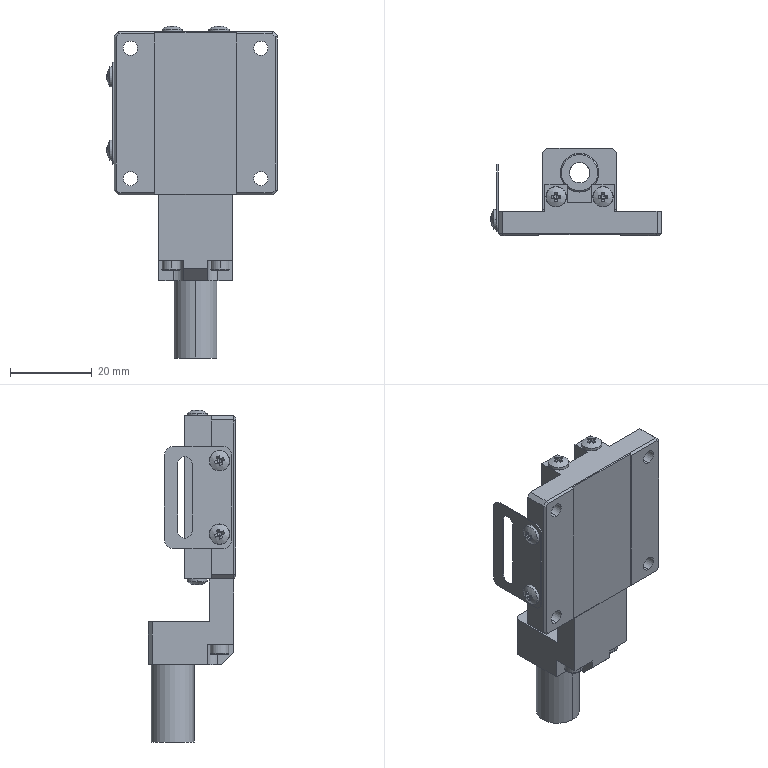Part | STEP file | Guide wheel mechanism revised.sldasm-Part-381 | 1 solid | 488 faces | box 41.75 x 21.5 x 81.45 mm | volume 18105 mm3 | plane 341 | cylinder 61 | cone 56 | spline 16 | torus 8 | sphere 6 | commonest cylinder face diameters 5 x16 3.5 x11 6.5 x8 2.5 x4 3 x4 4 x4